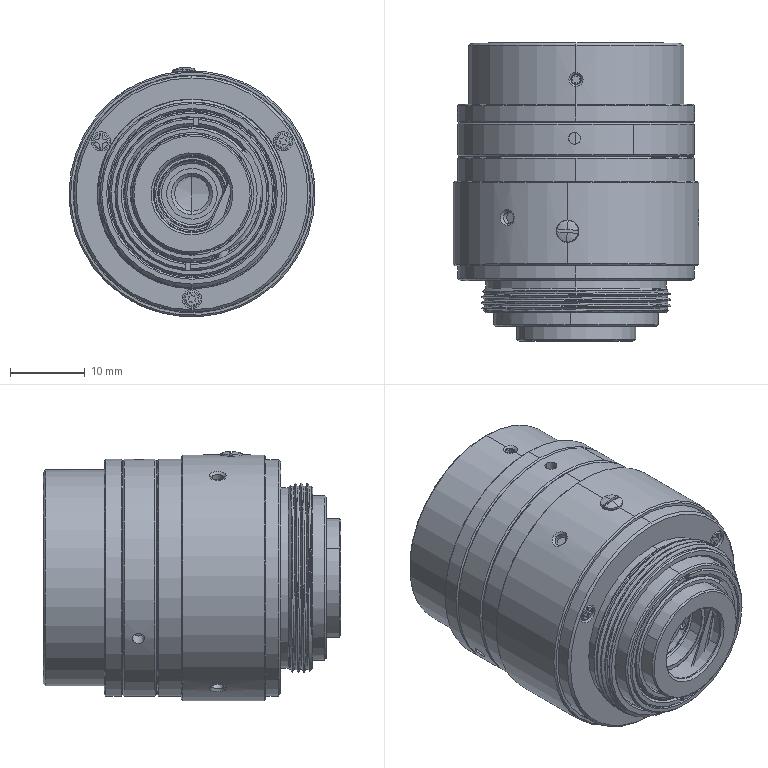Part | SolidWorks | features BaseBody 33 | 31 solids | 1222 faces | box 33 x 39.959 x 33.465 mm | volume 16722 mm3 | cylinder 447 | cone 318 | plane 268 | spline 169 | torus 12 | sphere 8 | commonest cylinder face diameters 0.6 x24 1.6 x22 2.6 x20 3 x19 1.2 x18 1.25 x16